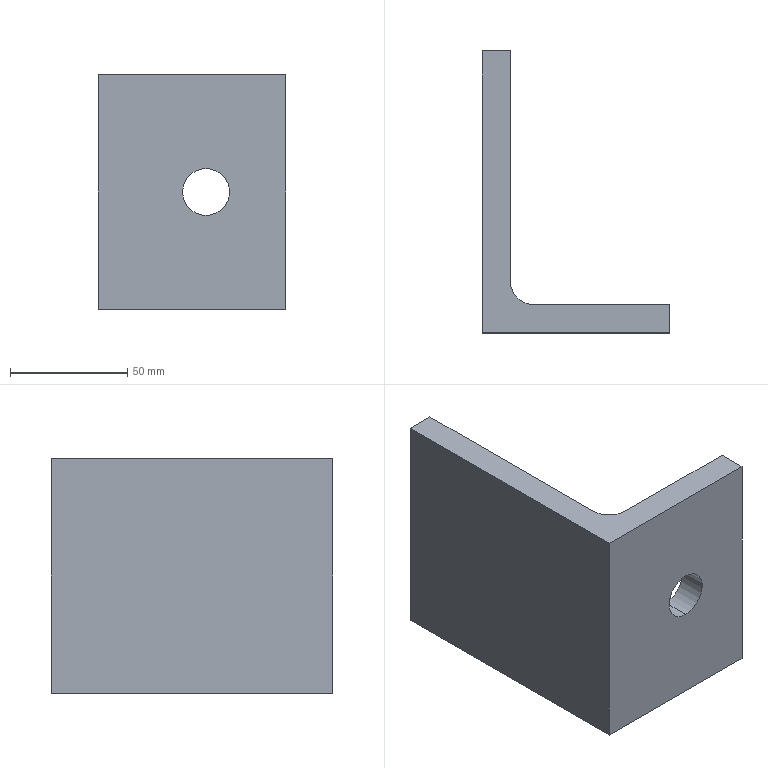Part | SolidWorks | features Extrusion 1, ICE 1 | 1 solid | 11 faces | box 80 x 120 x 100 mm | volume 223976 mm3 | plane 8 | cylinder 3 | commonest cylinder face diameters 20 x3
STEP:
#1=CARTESIAN_POINT('',(46.,-120.,40.));
#2=VERTEX_POINT('',#1);
#3=CARTESIAN_POINT('',(46.,-120.,60.));
#4=VERTEX_POINT('',#3);
#5=CARTESIAN_POINT('',(46.,-120.,50.));
#6=DIRECTION('',(0.,1.,0.));
#7=DIRECTION('',(0.,0.,1.));
#8=AXIS2_PLACEMENT_3D('',#5,#6,#7);
#9=CIRCLE('',#8,10.);
#10=EDGE_CURVE('',#2,#4,#9,.T.);
#11=ORIENTED_EDGE('',*,*,#10,.F.);
#12=CARTESIAN_POINT('',(46.,-108.,40.));
#13=VERTEX_POINT('',#12);
#14=CARTESIAN_POINT('',(46.,-208.,40.));
#15=DIRECTION('',(0.,1.,0.));
#16=VECTOR('',#15,1000.);
#17=LINE('',#14,#16);
#18=EDGE_CURVE('',#2,#13,#17,.T.);
#19=ORIENTED_EDGE('',*,*,#18,.T.);
#20=CARTESIAN_POINT('',(46.,-108.,60.));
#21=VERTEX_POINT('',#20);
#22=CARTESIAN_POINT('',(46.,-108.,50.));
#23=DIRECTION('',(0.,1.,0.));
#24=DIRECTION('',(0.,0.,1.));
#25=AXIS2_PLACEMENT_3D('',#22,#23,#24);
#26=CIRCLE('',#25,10.);
#27=EDGE_CURVE('',#13,#21,#26,.T.);
#28=ORIENTED_EDGE('',*,*,#27,.T.);
#29=CARTESIAN_POINT('',(46.,-208.,60.));
#30=DIRECTION('',(0.,1.,0.));
#31=VECTOR('',#30,1000.);
#32=LINE('',#29,#31);
#33=EDGE_CURVE('',#4,#21,#32,.T.);
#34=ORIENTED_EDGE('',*,*,#33,.F.);
#35=EDGE_LOOP('',(#11,#19,#28,#34));
#36=FACE_OUTER_BOUND('',#35,.T.);
#37=CARTESIAN_POINT('',(46.,-208.,50.));
#38=DIRECTION('',(0.,1.,0.));
#39=DIRECTION('',(0.,0.,1.));
#40=AXIS2_PLACEMENT_3D('',#37,#38,#39);
#41=CYLINDRICAL_SURFACE('',#40,10.);
#42=ADVANCED_FACE('',(#36),#41,.F.);
#43=CARTESIAN_POINT('',(46.,-108.,50.));
#44=DIRECTION('',(0.,1.,0.));
#45=DIRECTION('',(0.,0.,1.));
#46=AXIS2_PLACEMENT_3D('',#43,#44,#45);
#47=CIRCLE('',#46,10.);
#48=EDGE_CURVE('',#21,#13,#47,.T.);
#49=ORIENTED_EDGE('',*,*,#48,.F.);
#50=ORIENTED_EDGE('',*,*,#27,.F.);
#51=EDGE_LOOP('',(#49,#50));
#52=FACE_BOUND('',#51,.T.);
#53=CARTESIAN_POINT('',(22.,-108.,0.));
#54=VERTEX_POINT('',#53);
#55=CARTESIAN_POINT('',(80.,-108.,0.));
#56=VERTEX_POINT('',#55);
#57=CARTESIAN_POINT('',(22.,-108.,0.));
#58=DIRECTION('',(1.,0.,0.));
#59=VECTOR('',#58,1000.);
#60=LINE('',#57,#59);
#61=EDGE_CURVE('',#54,#56,#60,.T.);
#62=ORIENTED_EDGE('',*,*,#61,.F.);
#63=CARTESIAN_POINT('',(22.,-108.,100.));
#64=VERTEX_POINT('',#63);
#65=CARTESIAN_POINT('',(22.,-108.,100.));
#66=DIRECTION('',(0.,0.,-1.));
#67=VECTOR('',#66,1000.);
#68=LINE('',#65,#67);
#69=EDGE_CURVE('',#64,#54,#68,.T.);
#70=ORIENTED_EDGE('',*,*,#69,.F.);
#71=CARTESIAN_POINT('',(80.,-108.,100.));
#72=VERTEX_POINT('',#71);
#73=CARTESIAN_POINT('',(22.,-108.,100.));
#74=DIRECTION('',(1.,0.,0.));
#75=VECTOR('',#74,1000.);
#76=LINE('',#73,#75);
#77=EDGE_CURVE('',#64,#72,#76,.T.);
#78=ORIENTED_EDGE('',*,*,#77,.T.);
#79=CARTESIAN_POINT('',(80.,-108.,100.));
#80=DIRECTION('',(0.,0.,-1.));
#81=VECTOR('',#80,1000.);
#82=LINE('',#79,#81);
#83=EDGE_CURVE('',#72,#56,#82,.T.);
#84=ORIENTED_EDGE('',*,*,#83,.T.);
#85=EDGE_LOOP('',(#62,#70,#78,#84));
#86=FACE_OUTER_BOUND('',#85,.T.);
#87=CARTESIAN_POINT('',(22.,-108.,100.));
#88=DIRECTION('',(0.,1.,0.));
#89=DIRECTION('',(0.,0.,1.));
#90=AXIS2_PLACEMENT_3D('',#87,#88,#89);
#91=PLANE('',#90);
#92=ADVANCED_FACE('',(#52,#86),#91,.T.);
#93=CARTESIAN_POINT('',(12.,-98.,0.));
#94=VERTEX_POINT('',#93);
#95=CARTESIAN_POINT('',(22.,-98.,0.));
#96=DIRECTION('',(0.,0.,1.));
#97=DIRECTION('',(1.,0.,0.));
#98=AXIS2_PLACEMENT_3D('',#95,#96,#97);
#99=CIRCLE('',#98,10.);
#100=EDGE_CURVE('',#94,#54,#99,.T.);
#101=ORIENTED_EDGE('',*,*,#100,.F.);
#102=CARTESIAN_POINT('',(12.,-98.,100.));
#103=VERTEX_POINT('',#102);
#104=CARTESIAN_POINT('',(12.,-98.,100.));
#105=DIRECTION('',(0.,0.,-1.));
#106=VECTOR('',#105,1000.);
#107=LINE('',#104,#106);
#108=EDGE_CURVE('',#103,#94,#107,.T.);
#109=ORIENTED_EDGE('',*,*,#108,.F.);
#110=CARTESIAN_POINT('',(22.,-98.,100.));
#111=DIRECTION('',(0.,0.,1.));
#112=DIRECTION('',(1.,0.,0.));
#113=AXIS2_PLACEMENT_3D('',#110,#111,#112);
#114=CIRCLE('',#113,10.);
#115=EDGE_CURVE('',#103,#64,#114,.T.);
#116=ORIENTED_EDGE('',*,*,#115,.T.);
#117=ORIENTED_EDGE('',*,*,#69,.T.);
#118=EDGE_LOOP('',(#101,#109,#116,#117));
#119=FACE_OUTER_BOUND('',#118,.T.);
#120=CARTESIAN_POINT('',(22.,-98.,100.));
#121=DIRECTION('',(0.,0.,-1.));
#122=DIRECTION('',(-1.,0.,0.));
#123=AXIS2_PLACEMENT_3D('',#120,#121,#122);
#124=CYLINDRICAL_SURFACE('',#123,10.);
#125=ADVANCED_FACE('',(#119),#124,.F.);
#126=CARTESIAN_POINT('',(12.,0.,0.));
#127=VERTEX_POINT('',#126);
#128=CARTESIAN_POINT('',(12.,0.,0.));
#129=DIRECTION('',(0.,-1.,0.));
#130=VECTOR('',#129,1000.);
#131=LINE('',#128,#130);
#132=EDGE_CURVE('',#127,#94,#131,.T.);
#133=ORIENTED_EDGE('',*,*,#132,.F.);
#134=CARTESIAN_POINT('',(12.,0.,100.));
#135=VERTEX_POINT('',#134);
#136=CARTESIAN_POINT('',(12.,0.,100.));
#137=DIRECTION('',(0.,0.,-1.));
#138=VECTOR('',#137,1000.);
#139=LINE('',#136,#138);
#140=EDGE_CURVE('',#135,#127,#139,.T.);
#141=ORIENTED_EDGE('',*,*,#140,.F.);
#142=CARTESIAN_POINT('',(12.,0.,100.));
#143=DIRECTION('',(0.,-1.,0.));
#144=VECTOR('',#143,1000.);
#145=LINE('',#142,#144);
#146=EDGE_CURVE('',#135,#103,#145,.T.);
#147=ORIENTED_EDGE('',*,*,#146,.T.);
#148=ORIENTED_EDGE('',*,*,#108,.T.);
#149=EDGE_LOOP('',(#133,#141,#147,#148));
#150=FACE_OUTER_BOUND('',#149,.T.);
#151=CARTESIAN_POINT('',(12.,0.,100.));
#152=DIRECTION('',(1.,0.,0.));
#153=DIRECTION('',(0.,0.,-1.));
#154=AXIS2_PLACEMENT_3D('',#151,#152,#153);
#155=PLANE('',#154);
#156=ADVANCED_FACE('',(#150),#155,.T.);
#157=CARTESIAN_POINT('',(0.,0.,0.));
#158=VERTEX_POINT('',#157);
#159=CARTESIAN_POINT('',(12.,0.,0.));
#160=DIRECTION('',(-1.,0.,0.));
#161=VECTOR('',#160,1000.);
#162=LINE('',#159,#161);
#163=EDGE_CURVE('',#127,#158,#162,.T.);
#164=ORIENTED_EDGE('',*,*,#163,.T.);
#165=CARTESIAN_POINT('',(0.,0.,100.));
#166=VERTEX_POINT('',#165);
#167=CARTESIAN_POINT('',(0.,0.,100.));
#168=DIRECTION('',(0.,0.,-1.));
#169=VECTOR('',#168,1000.);
#170=LINE('',#167,#169);
#171=EDGE_CURVE('',#166,#158,#170,.T.);
#172=ORIENTED_EDGE('',*,*,#171,.F.);
#173=CARTESIAN_POINT('',(12.,0.,100.));
#174=DIRECTION('',(-1.,0.,0.));
#175=VECTOR('',#174,1000.);
#176=LINE('',#173,#175);
#177=EDGE_CURVE('',#135,#166,#176,.T.);
#178=ORIENTED_EDGE('',*,*,#177,.F.);
#179=ORIENTED_EDGE('',*,*,#140,.T.);
#180=EDGE_LOOP('',(#164,#172,#178,#179));
#181=FACE_OUTER_BOUND('',#180,.T.);
#182=CARTESIAN_POINT('',(12.,0.,100.));
#183=DIRECTION('',(0.,-1.,0.));
#184=DIRECTION('',(0.,0.,-1.));
#185=AXIS2_PLACEMENT_3D('',#182,#183,#184);
#186=PLANE('',#185);
#187=ADVANCED_FACE('',(#181),#186,.F.);
#188=CARTESIAN_POINT('',(0.,-120.,0.));
#189=VERTEX_POINT('',#188);
#190=CARTESIAN_POINT('',(0.,0.,0.));
#191=DIRECTION('',(0.,-1.,0.));
#192=VECTOR('',#191,1000.);
#193=LINE('',#190,#192);
#194=EDGE_CURVE('',#158,#189,#193,.T.);
#195=ORIENTED_EDGE('',*,*,#194,.T.);
#196=CARTESIAN_POINT('',(0.,-120.,100.));
#197=VERTEX_POINT('',#196);
#198=CARTESIAN_POINT('',(0.,-120.,100.));
#199=DIRECTION('',(0.,0.,-1.));
#200=VECTOR('',#199,1000.);
#201=LINE('',#198,#200);
#202=EDGE_CURVE('',#197,#189,#201,.T.);
#203=ORIENTED_EDGE('',*,*,#202,.F.);
#204=CARTESIAN_POINT('',(0.,0.,100.));
#205=DIRECTION('',(0.,-1.,0.));
#206=VECTOR('',#205,1000.);
#207=LINE('',#204,#206);
#208=EDGE_CURVE('',#166,#197,#207,.T.);
#209=ORIENTED_EDGE('',*,*,#208,.F.);
#210=ORIENTED_EDGE('',*,*,#171,.T.);
#211=EDGE_LOOP('',(#195,#203,#209,#210));
#212=FACE_OUTER_BOUND('',#211,.T.);
#213=CARTESIAN_POINT('',(0.,0.,100.));
#214=DIRECTION('',(1.,0.,0.));
#215=DIRECTION('',(0.,1.,0.));
#216=AXIS2_PLACEMENT_3D('',#213,#214,#215);
#217=PLANE('',#216);
#218=ADVANCED_FACE('',(#212),#217,.F.);
#219=CARTESIAN_POINT('',(46.,-120.,50.));
#220=DIRECTION('',(0.,1.,0.));
#221=DIRECTION('',(0.,0.,1.));
#222=AXIS2_PLACEMENT_3D('',#219,#220,#221);
#223=CIRCLE('',#222,10.);
#224=EDGE_CURVE('',#4,#2,#223,.T.);
#225=ORIENTED_EDGE('',*,*,#224,.T.);
#226=ORIENTED_EDGE('',*,*,#10,.T.);
#227=EDGE_LOOP('',(#225,#226));
#228=FACE_BOUND('',#227,.T.);
#229=CARTESIAN_POINT('',(80.,-120.,0.));
#230=VERTEX_POINT('',#229);
#231=CARTESIAN_POINT('',(0.,-120.,0.));
#232=DIRECTION('',(1.,0.,0.));
#233=VECTOR('',#232,1000.);
#234=LINE('',#231,#233);
#235=EDGE_CURVE('',#189,#230,#234,.T.);
#236=ORIENTED_EDGE('',*,*,#235,.T.);
#237=CARTESIAN_POINT('',(80.,-120.,100.));
#238=VERTEX_POINT('',#237);
#239=CARTESIAN_POINT('',(80.,-120.,100.));
#240=DIRECTION('',(0.,0.,-1.));
#241=VECTOR('',#240,1000.);
#242=LINE('',#239,#241);
#243=EDGE_CURVE('',#238,#230,#242,.T.);
#244=ORIENTED_EDGE('',*,*,#243,.F.);
#245=CARTESIAN_POINT('',(0.,-120.,100.));
#246=DIRECTION('',(1.,0.,0.));
#247=VECTOR('',#246,1000.);
#248=LINE('',#245,#247);
#249=EDGE_CURVE('',#197,#238,#248,.T.);
#250=ORIENTED_EDGE('',*,*,#249,.F.);
#251=ORIENTED_EDGE('',*,*,#202,.T.);
#252=EDGE_LOOP('',(#236,#244,#250,#251));
#253=FACE_OUTER_BOUND('',#252,.T.);
#254=CARTESIAN_POINT('',(0.,-120.,100.));
#255=DIRECTION('',(0.,1.,0.));
#256=DIRECTION('',(0.,0.,1.));
#257=AXIS2_PLACEMENT_3D('',#254,#255,#256);
#258=PLANE('',#257);
#259=ADVANCED_FACE('',(#228,#253),#258,.F.);
#260=CARTESIAN_POINT('',(80.,-108.,0.));
#261=DIRECTION('',(0.,-1.,0.));
#262=VECTOR('',#261,1000.);
#263=LINE('',#260,#262);
#264=EDGE_CURVE('',#56,#230,#263,.T.);
#265=ORIENTED_EDGE('',*,*,#264,.F.);
#266=ORIENTED_EDGE('',*,*,#83,.F.);
#267=CARTESIAN_POINT('',(80.,-108.,100.));
#268=DIRECTION('',(0.,-1.,0.));
#269=VECTOR('',#268,1000.);
#270=LINE('',#267,#269);
#271=EDGE_CURVE('',#72,#238,#270,.T.);
#272=ORIENTED_EDGE('',*,*,#271,.T.);
#273=ORIENTED_EDGE('',*,*,#243,.T.);
#274=EDGE_LOOP('',(#265,#266,#272,#273));
#275=FACE_OUTER_BOUND('',#274,.T.);
#276=CARTESIAN_POINT('',(80.,-108.,100.));
#277=DIRECTION('',(1.,0.,0.));
#278=DIRECTION('',(0.,0.,-1.));
#279=AXIS2_PLACEMENT_3D('',#276,#277,#278);
#280=PLANE('',#279);
#281=ADVANCED_FACE('',(#275),#280,.T.);
#282=ORIENTED_EDGE('',*,*,#77,.F.);
#283=ORIENTED_EDGE('',*,*,#115,.F.);
#284=ORIENTED_EDGE('',*,*,#146,.F.);
#285=ORIENTED_EDGE('',*,*,#177,.T.);
#286=ORIENTED_EDGE('',*,*,#208,.T.);
#287=ORIENTED_EDGE('',*,*,#249,.T.);
#288=ORIENTED_EDGE('',*,*,#271,.F.);
#289=EDGE_LOOP('',(#282,#283,#284,#285,#286,#287,#288));
#290=FACE_OUTER_BOUND('',#289,.T.);
#291=CARTESIAN_POINT('',(22.,-98.,100.));
#292=DIRECTION('',(0.,0.,1.));
#293=DIRECTION('',(1.,0.,0.));
#294=AXIS2_PLACEMENT_3D('',#291,#292,#293);
#295=PLANE('',#294);
#296=ADVANCED_FACE('',(#290),#295,.T.);
#297=ORIENTED_EDGE('',*,*,#61,.T.);
#298=ORIENTED_EDGE('',*,*,#264,.T.);
#299=ORIENTED_EDGE('',*,*,#235,.F.);
#300=ORIENTED_EDGE('',*,*,#194,.F.);
#301=ORIENTED_EDGE('',*,*,#163,.F.);
#302=ORIENTED_EDGE('',*,*,#132,.T.);
#303=ORIENTED_EDGE('',*,*,#100,.T.);
#304=EDGE_LOOP('',(#297,#298,#299,#300,#301,#302,#303));
#305=FACE_OUTER_BOUND('',#304,.T.);
#306=CARTESIAN_POINT('',(22.,-98.,0.));
#307=DIRECTION('',(0.,0.,1.));
#308=DIRECTION('',(1.,0.,0.));
#309=AXIS2_PLACEMENT_3D('',#306,#307,#308);
#310=PLANE('',#309);
#311=ADVANCED_FACE('',(#305),#310,.F.);
#312=ORIENTED_EDGE('',*,*,#18,.F.);
#313=ORIENTED_EDGE('',*,*,#224,.F.);
#314=ORIENTED_EDGE('',*,*,#33,.T.);
#315=ORIENTED_EDGE('',*,*,#48,.T.);
#316=EDGE_LOOP('',(#312,#313,#314,#315));
#317=FACE_OUTER_BOUND('',#316,.T.);
#318=CARTESIAN_POINT('',(46.,-208.,50.));
#319=DIRECTION('',(0.,1.,0.));
#320=DIRECTION('',(0.,0.,1.));
#321=AXIS2_PLACEMENT_3D('',#318,#319,#320);
#322=CYLINDRICAL_SURFACE('',#321,10.);
#323=ADVANCED_FACE('',(#317),#322,.F.);
#324=CLOSED_SHELL('',(#42,#92,#125,#156,#187,#218,#259,#281,#296,#311,#323));
#325=MANIFOLD_SOLID_BREP('',#324);
#326=CARTESIAN_POINT('',(0.,0.,0.));
#327=DIRECTION('',(0.,0.,1.));
#328=DIRECTION('',(1.,0.,0.));
#329=AXIS2_PLACEMENT_3D('',#326,#327,#328);
#330=(LENGTH_UNIT()NAMED_UNIT(*)SI_UNIT(.MILLI.,.METRE.));
#331=UNCERTAINTY_MEASURE_WITH_UNIT(LENGTH_MEASURE(0.00001),#330,'','');
#332=(NAMED_UNIT(*)PLANE_ANGLE_UNIT()SI_UNIT($,.RADIAN.));
#333=(NAMED_UNIT(*)SI_UNIT($,.STERADIAN.)SOLID_ANGLE_UNIT());
#334=(GEOMETRIC_REPRESENTATION_CONTEXT(3)GLOBAL_UNCERTAINTY_ASSIGNED_CONTEXT((#331))GLOBAL_UNIT_ASSIGNED_CONTEXT((#330,#332,#333))REPRESENTATION_CONTEXT('',''));
#335=ADVANCED_BREP_SHAPE_REPRESENTATION('',(#325,#329),#334);